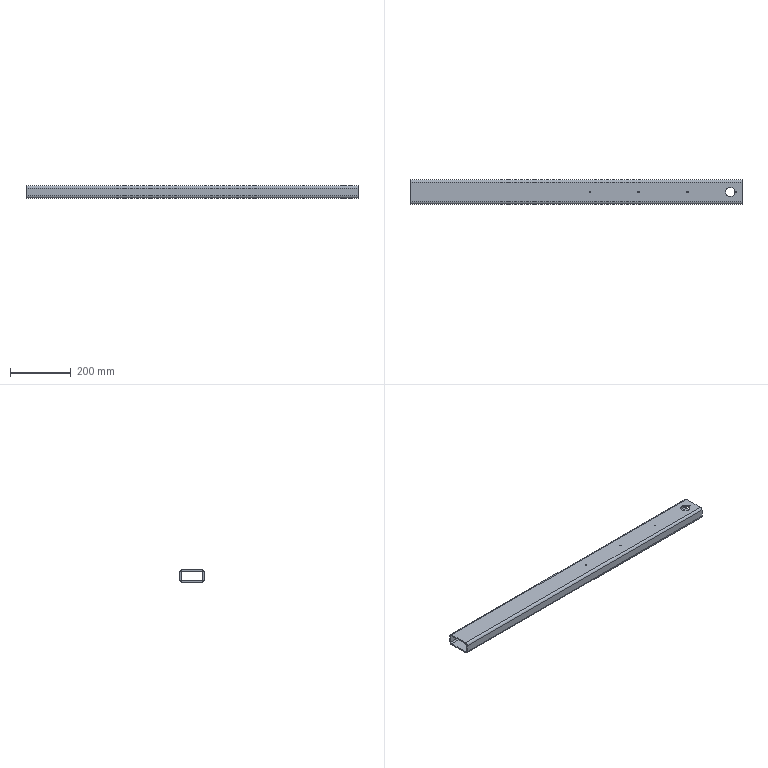Part | SolidWorks | features Cut 1, HoleWzd 1, WeldMemberFeat 1, WeldmentFeature 1 | 1 solid | 38 faces | box 1089 x 80 x 40 mm | volume 924590 mm3 | cylinder 28 | plane 10 | commonest cylinder face diameters 5 x16 8 x4 16 x4 30 x4
STEP:
#1=CARTESIAN_POINT('',(1036.,0.,-20.));
#2=VERTEX_POINT('',#1);
#3=CARTESIAN_POINT('',(1066.,0.,-20.));
#4=VERTEX_POINT('',#3);
#5=CARTESIAN_POINT('',(1051.,0.,-20.));
#6=DIRECTION('',(0.,0.,1.));
#7=DIRECTION('',(1.,0.,0.));
#8=AXIS2_PLACEMENT_3D('',#5,#6,#7);
#9=CIRCLE('',#8,15.);
#10=EDGE_CURVE('',#2,#4,#9,.T.);
#11=ORIENTED_EDGE('',*,*,#10,.F.);
#12=CARTESIAN_POINT('',(1036.,0.,-16.));
#13=VERTEX_POINT('',#12);
#14=CARTESIAN_POINT('',(1036.,0.,-20.));
#15=DIRECTION('',(0.,0.,1.));
#16=VECTOR('',#15,1000.);
#17=LINE('',#14,#16);
#18=EDGE_CURVE('',#2,#13,#17,.T.);
#19=ORIENTED_EDGE('',*,*,#18,.T.);
#20=CARTESIAN_POINT('',(1066.,0.,-16.));
#21=VERTEX_POINT('',#20);
#22=CARTESIAN_POINT('',(1051.,0.,-16.));
#23=DIRECTION('',(0.,0.,1.));
#24=DIRECTION('',(1.,0.,0.));
#25=AXIS2_PLACEMENT_3D('',#22,#23,#24);
#26=CIRCLE('',#25,15.);
#27=EDGE_CURVE('',#13,#21,#26,.T.);
#28=ORIENTED_EDGE('',*,*,#27,.T.);
#29=CARTESIAN_POINT('',(1066.,0.,-20.));
#30=DIRECTION('',(0.,0.,1.));
#31=VECTOR('',#30,1000.);
#32=LINE('',#29,#31);
#33=EDGE_CURVE('',#4,#21,#32,.T.);
#34=ORIENTED_EDGE('',*,*,#33,.F.);
#35=EDGE_LOOP('',(#11,#19,#28,#34));
#36=FACE_OUTER_BOUND('',#35,.T.);
#37=CARTESIAN_POINT('',(1051.,0.,-20.));
#38=DIRECTION('',(0.,0.,1.));
#39=DIRECTION('',(1.,0.,0.));
#40=AXIS2_PLACEMENT_3D('',#37,#38,#39);
#41=CYLINDRICAL_SURFACE('',#40,15.);
#42=ADVANCED_FACE('',(#36),#41,.F.);
#43=CARTESIAN_POINT('',(1066.,0.,16.));
#44=VERTEX_POINT('',#43);
#45=CARTESIAN_POINT('',(1036.,0.,16.));
#46=VERTEX_POINT('',#45);
#47=CARTESIAN_POINT('',(1051.,0.,16.));
#48=DIRECTION('',(0.,0.,-1.));
#49=DIRECTION('',(-1.,0.,0.));
#50=AXIS2_PLACEMENT_3D('',#47,#48,#49);
#51=CIRCLE('',#50,15.);
#52=EDGE_CURVE('',#44,#46,#51,.T.);
#53=ORIENTED_EDGE('',*,*,#52,.T.);
#54=CARTESIAN_POINT('',(1036.,0.,20.));
#55=VERTEX_POINT('',#54);
#56=CARTESIAN_POINT('',(1036.,0.,-20.));
#57=DIRECTION('',(0.,0.,1.));
#58=VECTOR('',#57,1000.);
#59=LINE('',#56,#58);
#60=EDGE_CURVE('',#46,#55,#59,.T.);
#61=ORIENTED_EDGE('',*,*,#60,.T.);
#62=CARTESIAN_POINT('',(1066.,0.,20.));
#63=VERTEX_POINT('',#62);
#64=CARTESIAN_POINT('',(1051.,0.,20.));
#65=DIRECTION('',(0.,0.,1.));
#66=DIRECTION('',(1.,0.,0.));
#67=AXIS2_PLACEMENT_3D('',#64,#65,#66);
#68=CIRCLE('',#67,15.);
#69=EDGE_CURVE('',#55,#63,#68,.T.);
#70=ORIENTED_EDGE('',*,*,#69,.T.);
#71=CARTESIAN_POINT('',(1066.,0.,-20.));
#72=DIRECTION('',(0.,0.,1.));
#73=VECTOR('',#72,1000.);
#74=LINE('',#71,#73);
#75=EDGE_CURVE('',#44,#63,#74,.T.);
#76=ORIENTED_EDGE('',*,*,#75,.F.);
#77=EDGE_LOOP('',(#53,#61,#70,#76));
#78=FACE_OUTER_BOUND('',#77,.T.);
#79=CARTESIAN_POINT('',(1051.,0.,-20.));
#80=DIRECTION('',(0.,0.,1.));
#81=DIRECTION('',(1.,0.,0.));
#82=AXIS2_PLACEMENT_3D('',#79,#80,#81);
#83=CYLINDRICAL_SURFACE('',#82,15.);
#84=ADVANCED_FACE('',(#78),#83,.F.);
#85=CARTESIAN_POINT('',(587.5,0.,-16.));
#86=VERTEX_POINT('',#85);
#87=CARTESIAN_POINT('',(592.5,0.,-16.));
#88=VERTEX_POINT('',#87);
#89=CARTESIAN_POINT('',(590.,0.,-16.));
#90=DIRECTION('',(0.,0.,1.));
#91=DIRECTION('',(1.,0.,0.));
#92=AXIS2_PLACEMENT_3D('',#89,#90,#91);
#93=CIRCLE('',#92,2.5);
#94=EDGE_CURVE('',#86,#88,#93,.T.);
#95=ORIENTED_EDGE('',*,*,#94,.T.);
#96=CARTESIAN_POINT('',(592.5,0.,-20.));
#97=VERTEX_POINT('',#96);
#98=CARTESIAN_POINT('',(592.5,0.,-20.));
#99=DIRECTION('',(0.,0.,-1.));
#100=VECTOR('',#99,1000.);
#101=LINE('',#98,#100);
#102=EDGE_CURVE('',#88,#97,#101,.T.);
#103=ORIENTED_EDGE('',*,*,#102,.T.);
#104=CARTESIAN_POINT('',(587.5,0.,-20.));
#105=VERTEX_POINT('',#104);
#106=CARTESIAN_POINT('',(590.,0.,-20.));
#107=DIRECTION('',(0.,0.,-1.));
#108=DIRECTION('',(-1.,0.,0.));
#109=AXIS2_PLACEMENT_3D('',#106,#107,#108);
#110=CIRCLE('',#109,2.5);
#111=EDGE_CURVE('',#97,#105,#110,.T.);
#112=ORIENTED_EDGE('',*,*,#111,.T.);
#113=CARTESIAN_POINT('',(587.5,0.,-20.));
#114=DIRECTION('',(0.,0.,-1.));
#115=VECTOR('',#114,1000.);
#116=LINE('',#113,#115);
#117=EDGE_CURVE('',#86,#105,#116,.T.);
#118=ORIENTED_EDGE('',*,*,#117,.F.);
#119=EDGE_LOOP('',(#95,#103,#112,#118));
#120=FACE_OUTER_BOUND('',#119,.T.);
#121=CARTESIAN_POINT('',(590.,0.,-20.));
#122=DIRECTION('',(0.,0.,-1.));
#123=DIRECTION('',(-1.,0.,0.));
#124=AXIS2_PLACEMENT_3D('',#121,#122,#123);
#125=CYLINDRICAL_SURFACE('',#124,2.5);
#126=ADVANCED_FACE('',(#120),#125,.F.);
#127=CARTESIAN_POINT('',(592.5,0.,20.));
#128=VERTEX_POINT('',#127);
#129=CARTESIAN_POINT('',(587.5,0.,20.));
#130=VERTEX_POINT('',#129);
#131=CARTESIAN_POINT('',(590.,0.,20.));
#132=DIRECTION('',(0.,0.,-1.));
#133=DIRECTION('',(-1.,0.,0.));
#134=AXIS2_PLACEMENT_3D('',#131,#132,#133);
#135=CIRCLE('',#134,2.5);
#136=EDGE_CURVE('',#128,#130,#135,.T.);
#137=ORIENTED_EDGE('',*,*,#136,.F.);
#138=CARTESIAN_POINT('',(592.5,0.,16.));
#139=VERTEX_POINT('',#138);
#140=CARTESIAN_POINT('',(592.5,0.,-20.));
#141=DIRECTION('',(0.,0.,-1.));
#142=VECTOR('',#141,1000.);
#143=LINE('',#140,#142);
#144=EDGE_CURVE('',#128,#139,#143,.T.);
#145=ORIENTED_EDGE('',*,*,#144,.T.);
#146=CARTESIAN_POINT('',(587.5,0.,16.));
#147=VERTEX_POINT('',#146);
#148=CARTESIAN_POINT('',(590.,0.,16.));
#149=DIRECTION('',(0.,0.,-1.));
#150=DIRECTION('',(-1.,0.,0.));
#151=AXIS2_PLACEMENT_3D('',#148,#149,#150);
#152=CIRCLE('',#151,2.5);
#153=EDGE_CURVE('',#139,#147,#152,.T.);
#154=ORIENTED_EDGE('',*,*,#153,.T.);
#155=CARTESIAN_POINT('',(587.5,0.,-20.));
#156=DIRECTION('',(0.,0.,-1.));
#157=VECTOR('',#156,1000.);
#158=LINE('',#155,#157);
#159=EDGE_CURVE('',#130,#147,#158,.T.);
#160=ORIENTED_EDGE('',*,*,#159,.F.);
#161=EDGE_LOOP('',(#137,#145,#154,#160));
#162=FACE_OUTER_BOUND('',#161,.T.);
#163=CARTESIAN_POINT('',(590.,0.,-20.));
#164=DIRECTION('',(0.,0.,-1.));
#165=DIRECTION('',(-1.,0.,0.));
#166=AXIS2_PLACEMENT_3D('',#163,#164,#165);
#167=CYLINDRICAL_SURFACE('',#166,2.5);
#168=ADVANCED_FACE('',(#162),#167,.F.);
#169=CARTESIAN_POINT('',(752.5,0.,20.));
#170=VERTEX_POINT('',#169);
#171=CARTESIAN_POINT('',(747.5,0.,20.));
#172=VERTEX_POINT('',#171);
#173=CARTESIAN_POINT('',(750.,0.,20.));
#174=DIRECTION('',(0.,0.,-1.));
#175=DIRECTION('',(-1.,0.,0.));
#176=AXIS2_PLACEMENT_3D('',#173,#174,#175);
#177=CIRCLE('',#176,2.5);
#178=EDGE_CURVE('',#170,#172,#177,.T.);
#179=ORIENTED_EDGE('',*,*,#178,.F.);
#180=CARTESIAN_POINT('',(752.5,0.,16.));
#181=VERTEX_POINT('',#180);
#182=CARTESIAN_POINT('',(752.5,0.,-20.));
#183=DIRECTION('',(0.,0.,-1.));
#184=VECTOR('',#183,1000.);
#185=LINE('',#182,#184);
#186=EDGE_CURVE('',#170,#181,#185,.T.);
#187=ORIENTED_EDGE('',*,*,#186,.T.);
#188=CARTESIAN_POINT('',(747.5,0.,16.));
#189=VERTEX_POINT('',#188);
#190=CARTESIAN_POINT('',(750.,0.,16.));
#191=DIRECTION('',(0.,0.,-1.));
#192=DIRECTION('',(-1.,0.,0.));
#193=AXIS2_PLACEMENT_3D('',#190,#191,#192);
#194=CIRCLE('',#193,2.5);
#195=EDGE_CURVE('',#181,#189,#194,.T.);
#196=ORIENTED_EDGE('',*,*,#195,.T.);
#197=CARTESIAN_POINT('',(747.5,0.,-20.));
#198=DIRECTION('',(0.,0.,-1.));
#199=VECTOR('',#198,1000.);
#200=LINE('',#197,#199);
#201=EDGE_CURVE('',#172,#189,#200,.T.);
#202=ORIENTED_EDGE('',*,*,#201,.F.);
#203=EDGE_LOOP('',(#179,#187,#196,#202));
#204=FACE_OUTER_BOUND('',#203,.T.);
#205=CARTESIAN_POINT('',(750.,0.,-20.));
#206=DIRECTION('',(0.,0.,-1.));
#207=DIRECTION('',(-1.,0.,0.));
#208=AXIS2_PLACEMENT_3D('',#205,#206,#207);
#209=CYLINDRICAL_SURFACE('',#208,2.5);
#210=ADVANCED_FACE('',(#204),#209,.F.);
#211=CARTESIAN_POINT('',(747.5,0.,-16.));
#212=VERTEX_POINT('',#211);
#213=CARTESIAN_POINT('',(752.5,0.,-16.));
#214=VERTEX_POINT('',#213);
#215=CARTESIAN_POINT('',(750.,0.,-16.));
#216=DIRECTION('',(0.,0.,1.));
#217=DIRECTION('',(1.,0.,0.));
#218=AXIS2_PLACEMENT_3D('',#215,#216,#217);
#219=CIRCLE('',#218,2.5);
#220=EDGE_CURVE('',#212,#214,#219,.T.);
#221=ORIENTED_EDGE('',*,*,#220,.T.);
#222=CARTESIAN_POINT('',(752.5,0.,-20.));
#223=VERTEX_POINT('',#222);
#224=CARTESIAN_POINT('',(752.5,0.,-20.));
#225=DIRECTION('',(0.,0.,-1.));
#226=VECTOR('',#225,1000.);
#227=LINE('',#224,#226);
#228=EDGE_CURVE('',#214,#223,#227,.T.);
#229=ORIENTED_EDGE('',*,*,#228,.T.);
#230=CARTESIAN_POINT('',(747.5,0.,-20.));
#231=VERTEX_POINT('',#230);
#232=CARTESIAN_POINT('',(750.,0.,-20.));
#233=DIRECTION('',(0.,0.,-1.));
#234=DIRECTION('',(-1.,0.,0.));
#235=AXIS2_PLACEMENT_3D('',#232,#233,#234);
#236=CIRCLE('',#235,2.5);
#237=EDGE_CURVE('',#223,#231,#236,.T.);
#238=ORIENTED_EDGE('',*,*,#237,.T.);
#239=CARTESIAN_POINT('',(747.5,0.,-20.));
#240=DIRECTION('',(0.,0.,-1.));
#241=VECTOR('',#240,1000.);
#242=LINE('',#239,#241);
#243=EDGE_CURVE('',#212,#231,#242,.T.);
#244=ORIENTED_EDGE('',*,*,#243,.F.);
#245=EDGE_LOOP('',(#221,#229,#238,#244));
#246=FACE_OUTER_BOUND('',#245,.T.);
#247=CARTESIAN_POINT('',(750.,0.,-20.));
#248=DIRECTION('',(0.,0.,-1.));
#249=DIRECTION('',(-1.,0.,0.));
#250=AXIS2_PLACEMENT_3D('',#247,#248,#249);
#251=CYLINDRICAL_SURFACE('',#250,2.5);
#252=ADVANCED_FACE('',(#246),#251,.F.);
#253=CARTESIAN_POINT('',(907.5,0.,-16.));
#254=VERTEX_POINT('',#253);
#255=CARTESIAN_POINT('',(912.5,0.,-16.));
#256=VERTEX_POINT('',#255);
#257=CARTESIAN_POINT('',(910.,0.,-16.));
#258=DIRECTION('',(0.,0.,1.));
#259=DIRECTION('',(1.,0.,0.));
#260=AXIS2_PLACEMENT_3D('',#257,#258,#259);
#261=CIRCLE('',#260,2.5);
#262=EDGE_CURVE('',#254,#256,#261,.T.);
#263=ORIENTED_EDGE('',*,*,#262,.T.);
#264=CARTESIAN_POINT('',(912.5,0.,-20.));
#265=VERTEX_POINT('',#264);
#266=CARTESIAN_POINT('',(912.5,0.,-20.));
#267=DIRECTION('',(0.,0.,-1.));
#268=VECTOR('',#267,1000.);
#269=LINE('',#266,#268);
#270=EDGE_CURVE('',#256,#265,#269,.T.);
#271=ORIENTED_EDGE('',*,*,#270,.T.);
#272=CARTESIAN_POINT('',(907.5,0.,-20.));
#273=VERTEX_POINT('',#272);
#274=CARTESIAN_POINT('',(910.,0.,-20.));
#275=DIRECTION('',(0.,0.,-1.));
#276=DIRECTION('',(-1.,0.,0.));
#277=AXIS2_PLACEMENT_3D('',#274,#275,#276);
#278=CIRCLE('',#277,2.5);
#279=EDGE_CURVE('',#265,#273,#278,.T.);
#280=ORIENTED_EDGE('',*,*,#279,.T.);
#281=CARTESIAN_POINT('',(907.5,0.,-20.));
#282=DIRECTION('',(0.,0.,-1.));
#283=VECTOR('',#282,1000.);
#284=LINE('',#281,#283);
#285=EDGE_CURVE('',#254,#273,#284,.T.);
#286=ORIENTED_EDGE('',*,*,#285,.F.);
#287=EDGE_LOOP('',(#263,#271,#280,#286));
#288=FACE_OUTER_BOUND('',#287,.T.);
#289=CARTESIAN_POINT('',(910.,0.,-20.));
#290=DIRECTION('',(0.,0.,-1.));
#291=DIRECTION('',(-1.,0.,0.));
#292=AXIS2_PLACEMENT_3D('',#289,#290,#291);
#293=CYLINDRICAL_SURFACE('',#292,2.5);
#294=ADVANCED_FACE('',(#288),#293,.F.);
#295=CARTESIAN_POINT('',(912.5,0.,20.));
#296=VERTEX_POINT('',#295);
#297=CARTESIAN_POINT('',(907.5,0.,20.));
#298=VERTEX_POINT('',#297);
#299=CARTESIAN_POINT('',(910.,0.,20.));
#300=DIRECTION('',(0.,0.,-1.));
#301=DIRECTION('',(-1.,0.,0.));
#302=AXIS2_PLACEMENT_3D('',#299,#300,#301);
#303=CIRCLE('',#302,2.5);
#304=EDGE_CURVE('',#296,#298,#303,.T.);
#305=ORIENTED_EDGE('',*,*,#304,.F.);
#306=CARTESIAN_POINT('',(912.5,0.,16.));
#307=VERTEX_POINT('',#306);
#308=CARTESIAN_POINT('',(912.5,0.,-20.));
#309=DIRECTION('',(0.,0.,-1.));
#310=VECTOR('',#309,1000.);
#311=LINE('',#308,#310);
#312=EDGE_CURVE('',#296,#307,#311,.T.);
#313=ORIENTED_EDGE('',*,*,#312,.T.);
#314=CARTESIAN_POINT('',(907.5,0.,16.));
#315=VERTEX_POINT('',#314);
#316=CARTESIAN_POINT('',(910.,0.,16.));
#317=DIRECTION('',(0.,0.,-1.));
#318=DIRECTION('',(-1.,0.,0.));
#319=AXIS2_PLACEMENT_3D('',#316,#317,#318);
#320=CIRCLE('',#319,2.5);
#321=EDGE_CURVE('',#307,#315,#320,.T.);
#322=ORIENTED_EDGE('',*,*,#321,.T.);
#323=CARTESIAN_POINT('',(907.5,0.,-20.));
#324=DIRECTION('',(0.,0.,-1.));
#325=VECTOR('',#324,1000.);
#326=LINE('',#323,#325);
#327=EDGE_CURVE('',#298,#315,#326,.T.);
#328=ORIENTED_EDGE('',*,*,#327,.F.);
#329=EDGE_LOOP('',(#305,#313,#322,#328));
#330=FACE_OUTER_BOUND('',#329,.T.);
#331=CARTESIAN_POINT('',(910.,0.,-20.));
#332=DIRECTION('',(0.,0.,-1.));
#333=DIRECTION('',(-1.,0.,0.));
#334=AXIS2_PLACEMENT_3D('',#331,#332,#333);
#335=CYLINDRICAL_SURFACE('',#334,2.5);
#336=ADVANCED_FACE('',(#330),#335,.F.);
#337=CARTESIAN_POINT('',(1072.5,0.,20.));
#338=VERTEX_POINT('',#337);
#339=CARTESIAN_POINT('',(1067.5,0.,20.));
#340=VERTEX_POINT('',#339);
#341=CARTESIAN_POINT('',(1070.,0.,20.));
#342=DIRECTION('',(0.,0.,-1.));
#343=DIRECTION('',(-1.,0.,0.));
#344=AXIS2_PLACEMENT_3D('',#341,#342,#343);
#345=CIRCLE('',#344,2.5);
#346=EDGE_CURVE('',#338,#340,#345,.T.);
#347=ORIENTED_EDGE('',*,*,#346,.F.);
#348=CARTESIAN_POINT('',(1072.5,0.,16.));
#349=VERTEX_POINT('',#348);
#350=CARTESIAN_POINT('',(1072.5,0.,-20.));
#351=DIRECTION('',(0.,0.,-1.));
#352=VECTOR('',#351,1000.);
#353=LINE('',#350,#352);
#354=EDGE_CURVE('',#338,#349,#353,.T.);
#355=ORIENTED_EDGE('',*,*,#354,.T.);
#356=CARTESIAN_POINT('',(1067.5,0.,16.));
#357=VERTEX_POINT('',#356);
#358=CARTESIAN_POINT('',(1070.,0.,16.));
#359=DIRECTION('',(0.,0.,-1.));
#360=DIRECTION('',(-1.,0.,0.));
#361=AXIS2_PLACEMENT_3D('',#358,#359,#360);
#362=CIRCLE('',#361,2.5);
#363=EDGE_CURVE('',#349,#357,#362,.T.);
#364=ORIENTED_EDGE('',*,*,#363,.T.);
#365=CARTESIAN_POINT('',(1067.5,0.,-20.));
#366=DIRECTION('',(0.,0.,-1.));
#367=VECTOR('',#366,1000.);
#368=LINE('',#365,#367);
#369=EDGE_CURVE('',#340,#357,#368,.T.);
#370=ORIENTED_EDGE('',*,*,#369,.F.);
#371=EDGE_LOOP('',(#347,#355,#364,#370));
#372=FACE_OUTER_BOUND('',#371,.T.);
#373=CARTESIAN_POINT('',(1070.,0.,-20.));
#374=DIRECTION('',(0.,0.,-1.));
#375=DIRECTION('',(-1.,0.,0.));
#376=AXIS2_PLACEMENT_3D('',#373,#374,#375);
#377=CYLINDRICAL_SURFACE('',#376,2.5);
#378=ADVANCED_FACE('',(#372),#377,.F.);
#379=CARTESIAN_POINT('',(1067.5,0.,-16.));
#380=VERTEX_POINT('',#379);
#381=CARTESIAN_POINT('',(1072.5,0.,-16.));
#382=VERTEX_POINT('',#381);
#383=CARTESIAN_POINT('',(1070.,0.,-16.));
#384=DIRECTION('',(0.,0.,1.));
#385=DIRECTION('',(1.,0.,0.));
#386=AXIS2_PLACEMENT_3D('',#383,#384,#385);
#387=CIRCLE('',#386,2.5);
#388=EDGE_CURVE('',#380,#382,#387,.T.);
#389=ORIENTED_EDGE('',*,*,#388,.T.);
#390=CARTESIAN_POINT('',(1072.5,0.,-20.));
#391=VERTEX_POINT('',#390);
#392=CARTESIAN_POINT('',(1072.5,0.,-20.));
#393=DIRECTION('',(0.,0.,-1.));
#394=VECTOR('',#393,1000.);
#395=LINE('',#392,#394);
#396=EDGE_CURVE('',#382,#391,#395,.T.);
#397=ORIENTED_EDGE('',*,*,#396,.T.);
#398=CARTESIAN_POINT('',(1067.5,0.,-20.));
#399=VERTEX_POINT('',#398);
#400=CARTESIAN_POINT('',(1070.,0.,-20.));
#401=DIRECTION('',(0.,0.,-1.));
#402=DIRECTION('',(-1.,0.,0.));
#403=AXIS2_PLACEMENT_3D('',#400,#401,#402);
#404=CIRCLE('',#403,2.5);
#405=EDGE_CURVE('',#391,#399,#404,.T.);
#406=ORIENTED_EDGE('',*,*,#405,.T.);
#407=CARTESIAN_POINT('',(1067.5,0.,-20.));
#408=DIRECTION('',(0.,0.,-1.));
#409=VECTOR('',#408,1000.);
#410=LINE('',#407,#409);
#411=EDGE_CURVE('',#380,#399,#410,.T.);
#412=ORIENTED_EDGE('',*,*,#411,.F.);
#413=EDGE_LOOP('',(#389,#397,#406,#412));
#414=FACE_OUTER_BOUND('',#413,.T.);
#415=CARTESIAN_POINT('',(1070.,0.,-20.));
#416=DIRECTION('',(0.,0.,-1.));
#417=DIRECTION('',(-1.,0.,0.));
#418=AXIS2_PLACEMENT_3D('',#415,#416,#417);
#419=CYLINDRICAL_SURFACE('',#418,2.5);
#420=ADVANCED_FACE('',(#414),#419,.F.);
#421=CARTESIAN_POINT('',(1051.,0.,-20.));
#422=DIRECTION('',(0.,0.,1.));
#423=DIRECTION('',(1.,0.,0.));
#424=AXIS2_PLACEMENT_3D('',#421,#422,#423);
#425=CIRCLE('',#424,15.);
#426=EDGE_CURVE('',#4,#2,#425,.T.);
#427=ORIENTED_EDGE('',*,*,#426,.T.);
#428=ORIENTED_EDGE('',*,*,#10,.T.);
#429=EDGE_LOOP('',(#427,#428));
#430=FACE_BOUND('',#429,.T.);
#431=CARTESIAN_POINT('',(750.,0.,-20.));
#432=DIRECTION('',(0.,0.,-1.));
#433=DIRECTION('',(-1.,0.,0.));
#434=AXIS2_PLACEMENT_3D('',#431,#432,#433);
#435=CIRCLE('',#434,2.5);
#436=EDGE_CURVE('',#231,#223,#435,.T.);
#437=ORIENTED_EDGE('',*,*,#436,.F.);
#438=ORIENTED_EDGE('',*,*,#237,.F.);
#439=EDGE_LOOP('',(#437,#438));
#440=FACE_BOUND('',#439,.T.);
#441=CARTESIAN_POINT('',(910.,0.,-20.));
#442=DIRECTION('',(0.,0.,-1.));
#443=DIRECTION('',(-1.,0.,0.));
#444=AXIS2_PLACEMENT_3D('',#441,#442,#443);
#445=CIRCLE('',#444,2.5);
#446=EDGE_CURVE('',#273,#265,#445,.T.);
#447=ORIENTED_EDGE('',*,*,#446,.F.);
#448=ORIENTED_EDGE('',*,*,#279,.F.);
#449=EDGE_LOOP('',(#447,#448));
#450=FACE_BOUND('',#449,.T.);
#451=CARTESIAN_POINT('',(1070.,0.,-20.));
#452=DIRECTION('',(0.,0.,-1.));
#453=DIRECTION('',(-1.,0.,0.));
#454=AXIS2_PLACEMENT_3D('',#451,#452,#453);
#455=CIRCLE('',#454,2.5);
#456=EDGE_CURVE('',#399,#391,#455,.T.);
#457=ORIENTED_EDGE('',*,*,#456,.F.);
#458=ORIENTED_EDGE('',*,*,#405,.F.);
#459=EDGE_LOOP('',(#457,#458));
#460=FACE_BOUND('',#459,.T.);
#461=CARTESIAN_POINT('',(0.,-32.,-20.));
#462=VERTEX_POINT('',#461);
#463=CARTESIAN_POINT('',(0.,32.,-20.));
#464=VERTEX_POINT('',#463);
#465=CARTESIAN_POINT('',(0.,32.,-20.));
#466=DIRECTION('',(0.,1.,0.));
#467=VECTOR('',#466,1000.);
#468=LINE('',#465,#467);
#469=EDGE_CURVE('',#462,#464,#468,.T.);
#470=ORIENTED_EDGE('',*,*,#469,.T.);
#471=CARTESIAN_POINT('',(1089.,32.,-20.));
#472=VERTEX_POINT('',#471);
#473=CARTESIAN_POINT('',(1089.,32.,-20.));
#474=DIRECTION('',(-1.,0.,0.));
#475=VECTOR('',#474,1000.);
#476=LINE('',#473,#475);
#477=EDGE_CURVE('',#472,#464,#476,.T.);
#478=ORIENTED_EDGE('',*,*,#477,.F.);
#479=CARTESIAN_POINT('',(1089.,-32.,-20.));
#480=VERTEX_POINT('',#479);
#481=CARTESIAN_POINT('',(1089.,32.,-20.));
#482=DIRECTION('',(0.,1.,0.));
#483=VECTOR('',#482,1000.);
#484=LINE('',#481,#483);
#485=EDGE_CURVE('',#480,#472,#484,.T.);
#486=ORIENTED_EDGE('',*,*,#485,.F.);
#487=CARTESIAN_POINT('',(1089.,-32.,-20.));
#488=DIRECTION('',(-1.,0.,0.));
#489=VECTOR('',#488,1000.);
#490=LINE('',#487,#489);
#491=EDGE_CURVE('',#480,#462,#490,.T.);
#492=ORIENTED_EDGE('',*,*,#491,.T.);
#493=EDGE_LOOP('',(#470,#478,#486,#492));
#494=FACE_OUTER_BOUND('',#493,.T.);
#495=CARTESIAN_POINT('',(590.,0.,-20.));
#496=DIRECTION('',(0.,0.,-1.));
#497=DIRECTION('',(-1.,0.,0.));
#498=AXIS2_PLACEMENT_3D('',#495,#496,#497);
#499=CIRCLE('',#498,2.5);
#500=EDGE_CURVE('',#105,#97,#499,.T.);
#501=ORIENTED_EDGE('',*,*,#500,.F.);
#502=ORIENTED_EDGE('',*,*,#111,.F.);
#503=EDGE_LOOP('',(#501,#502));
#504=FACE_BOUND('',#503,.T.);
#505=CARTESIAN_POINT('',(1089.,32.,-20.));
#506=DIRECTION('',(0.,0.,1.));
#507=DIRECTION('',(1.,0.,0.));
#508=AXIS2_PLACEMENT_3D('',#505,#506,#507);
#509=PLANE('',#508);
#510=ADVANCED_FACE('',(#430,#440,#450,#460,#494,#504),#509,.F.);
#511=CARTESIAN_POINT('',(0.,40.,-12.));
#512=VERTEX_POINT('',#511);
#513=CARTESIAN_POINT('',(0.,32.,-12.));
#514=DIRECTION('',(1.,0.,0.));
#515=DIRECTION('',(0.,0.,-1.));
#516=AXIS2_PLACEMENT_3D('',#513,#514,#515);
#517=CIRCLE('',#516,8.);
#518=EDGE_CURVE('',#464,#512,#517,.T.);
#519=ORIENTED_EDGE('',*,*,#518,.T.);
#520=CARTESIAN_POINT('',(1089.,40.,-12.));
#521=VERTEX_POINT('',#520);
#522=CARTESIAN_POINT('',(1089.,40.,-12.));
#523=DIRECTION('',(-1.,0.,0.));
#524=VECTOR('',#523,1000.);
#525=LINE('',#522,#524);
#526=EDGE_CURVE('',#521,#512,#525,.T.);
#527=ORIENTED_EDGE('',*,*,#526,.F.);
#528=CARTESIAN_POINT('',(1089.,32.,-12.));
#529=DIRECTION('',(1.,0.,0.));
#530=DIRECTION('',(0.,0.,-1.));
#531=AXIS2_PLACEMENT_3D('',#528,#529,#530);
#532=CIRCLE('',#531,8.);
#533=EDGE_CURVE('',#472,#521,#532,.T.);
#534=ORIENTED_EDGE('',*,*,#533,.F.);
#535=ORIENTED_EDGE('',*,*,#477,.T.);
#536=EDGE_LOOP('',(#519,#527,#534,#535));
#537=FACE_OUTER_BOUND('',#536,.T.);
#538=CARTESIAN_POINT('',(1089.,32.,-12.));
#539=DIRECTION('',(-1.,0.,0.));
#540=DIRECTION('',(0.,0.,1.));
#541=AXIS2_PLACEMENT_3D('',#538,#539,#540);
#542=CYLINDRICAL_SURFACE('',#541,8.);
#543=ADVANCED_FACE('',(#537),#542,.T.);
#544=CARTESIAN_POINT('',(0.,40.,12.));
#545=VERTEX_POINT('',#544);
#546=CARTESIAN_POINT('',(0.,40.,-12.));
#547=DIRECTION('',(0.,0.,1.));
#548=VECTOR('',#547,1000.);
#549=LINE('',#546,#548);
#550=EDGE_CURVE('',#512,#545,#549,.T.);
#551=ORIENTED_EDGE('',*,*,#550,.T.);
#552=CARTESIAN_POINT('',(1089.,40.,12.));
#553=VERTEX_POINT('',#552);
#554=CARTESIAN_POINT('',(1089.,40.,12.));
#555=DIRECTION('',(-1.,0.,0.));
#556=VECTOR('',#555,1000.);
#557=LINE('',#554,#556);
#558=EDGE_CURVE('',#553,#545,#557,.T.);
#559=ORIENTED_EDGE('',*,*,#558,.F.);
#560=CARTESIAN_POINT('',(1089.,40.,-12.));
#561=DIRECTION('',(0.,0.,1.));
#562=VECTOR('',#561,1000.);
#563=LINE('',#560,#562);
#564=EDGE_CURVE('',#521,#553,#563,.T.);
#565=ORIENTED_EDGE('',*,*,#564,.F.);
#566=ORIENTED_EDGE('',*,*,#526,.T.);
#567=EDGE_LOOP('',(#551,#559,#565,#566));
#568=FACE_OUTER_BOUND('',#567,.T.);
#569=CARTESIAN_POINT('',(1089.,40.,-12.));
#570=DIRECTION('',(0.,-1.,0.));
#571=DIRECTION('',(0.,0.,-1.));
#572=AXIS2_PLACEMENT_3D('',#569,#570,#571);
#573=PLANE('',#572);
#574=ADVANCED_FACE('',(#568),#573,.F.);
#575=CARTESIAN_POINT('',(0.,32.,20.));
#576=VERTEX_POINT('',#575);
#577=CARTESIAN_POINT('',(0.,32.,12.));
#578=DIRECTION('',(1.,0.,0.));
#579=DIRECTION('',(0.,0.,-1.));
#580=AXIS2_PLACEMENT_3D('',#577,#578,#579);
#581=CIRCLE('',#580,8.);
#582=EDGE_CURVE('',#545,#576,#581,.T.);
#583=ORIENTED_EDGE('',*,*,#582,.T.);
#584=CARTESIAN_POINT('',(1089.,32.,20.));
#585=VERTEX_POINT('',#584);
#586=CARTESIAN_POINT('',(1089.,32.,20.));
#587=DIRECTION('',(-1.,0.,0.));
#588=VECTOR('',#587,1000.);
#589=LINE('',#586,#588);
#590=EDGE_CURVE('',#585,#576,#589,.T.);
#591=ORIENTED_EDGE('',*,*,#590,.F.);
#592=CARTESIAN_POINT('',(1089.,32.,12.));
#593=DIRECTION('',(1.,0.,0.));
#594=DIRECTION('',(0.,0.,-1.));
#595=AXIS2_PLACEMENT_3D('',#592,#593,#594);
#596=CIRCLE('',#595,8.);
#597=EDGE_CURVE('',#553,#585,#596,.T.);
#598=ORIENTED_EDGE('',*,*,#597,.F.);
#599=ORIENTED_EDGE('',*,*,#558,.T.);
#600=EDGE_LOOP('',(#583,#591,#598,#599));
#601=FACE_OUTER_BOUND('',#600,.T.);
#602=CARTESIAN_POINT('',(1089.,32.,12.));
#603=DIRECTION('',(-1.,0.,0.));
#604=DIRECTION('',(0.,0.,1.));
#605=AXIS2_PLACEMENT_3D('',#602,#603,#604);
#606=CYLINDRICAL_SURFACE('',#605,8.);
#607=ADVANCED_FACE('',(#601),#606,.T.);
#608=CARTESIAN_POINT('',(1051.,0.,20.));
#609=DIRECTION('',(0.,0.,1.));
#610=DIRECTION('',(1.,0.,0.));
#611=AXIS2_PLACEMENT_3D('',#608,#609,#610);
#612=CIRCLE('',#611,15.);
#613=EDGE_CURVE('',#63,#55,#612,.T.);
#614=ORIENTED_EDGE('',*,*,#613,.F.);
#615=ORIENTED_EDGE('',*,*,#69,.F.);
#616=EDGE_LOOP('',(#614,#615));
#617=FACE_BOUND('',#616,.T.);
#618=CARTESIAN_POINT('',(590.,0.,20.));
#619=DIRECTION('',(0.,0.,-1.));
#620=DIRECTION('',(-1.,0.,0.));
#621=AXIS2_PLACEMENT_3D('',#618,#619,#620);
#622=CIRCLE('',#621,2.5);
#623=EDGE_CURVE('',#130,#128,#622,.T.);
#624=ORIENTED_EDGE('',*,*,#623,.T.);
#625=ORIENTED_EDGE('',*,*,#136,.T.);
#626=EDGE_LOOP('',(#624,#625));
#627=FACE_BOUND('',#626,.T.);
#628=CARTESIAN_POINT('',(750.,0.,20.));
#629=DIRECTION('',(0.,0.,-1.));
#630=DIRECTION('',(-1.,0.,0.));
#631=AXIS2_PLACEMENT_3D('',#628,#629,#630);
#632=CIRCLE('',#631,2.5);
#633=EDGE_CURVE('',#172,#170,#632,.T.);
#634=ORIENTED_EDGE('',*,*,#633,.T.);
#635=ORIENTED_EDGE('',*,*,#178,.T.);
#636=EDGE_LOOP('',(#634,#635));
#637=FACE_BOUND('',#636,.T.);
#638=CARTESIAN_POINT('',(910.,0.,20.));
#639=DIRECTION('',(0.,0.,-1.));
#640=DIRECTION('',(-1.,0.,0.));
#641=AXIS2_PLACEMENT_3D('',#638,#639,#640);
#642=CIRCLE('',#641,2.5);
#643=EDGE_CURVE('',#298,#296,#642,.T.);
#644=ORIENTED_EDGE('',*,*,#643,.T.);
#645=ORIENTED_EDGE('',*,*,#304,.T.);
#646=EDGE_LOOP('',(#644,#645));
#647=FACE_BOUND('',#646,.T.);
#648=CARTESIAN_POINT('',(1070.,0.,20.));
#649=DIRECTION('',(0.,0.,-1.));
#650=DIRECTION('',(-1.,0.,0.));
#651=AXIS2_PLACEMENT_3D('',#648,#649,#650);
#652=CIRCLE('',#651,2.5);
#653=EDGE_CURVE('',#340,#338,#652,.T.);
#654=ORIENTED_EDGE('',*,*,#653,.T.);
#655=ORIENTED_EDGE('',*,*,#346,.T.);
#656=EDGE_LOOP('',(#654,#655));
#657=FACE_BOUND('',#656,.T.);
#658=CARTESIAN_POINT('',(0.,-32.,20.));
#659=VERTEX_POINT('',#658);
#660=CARTESIAN_POINT('',(0.,-32.,20.));
#661=DIRECTION('',(0.,-1.,0.));
#662=VECTOR('',#661,1000.);
#663=LINE('',#660,#662);
#664=EDGE_CURVE('',#576,#659,#663,.T.);
#665=ORIENTED_EDGE('',*,*,#664,.T.);
#666=CARTESIAN_POINT('',(1089.,-32.,20.));
#667=VERTEX_POINT('',#666);
#668=CARTESIAN_POINT('',(1089.,-32.,20.));
#669=DIRECTION('',(-1.,0.,0.));
#670=VECTOR('',#669,1000.);
#671=LINE('',#668,#670);
#672=EDGE_CURVE('',#667,#659,#671,.T.);
#673=ORIENTED_EDGE('',*,*,#672,.F.);
#674=CARTESIAN_POINT('',(1089.,-32.,20.));
#675=DIRECTION('',(0.,-1.,0.));
#676=VECTOR('',#675,1000.);
#677=LINE('',#674,#676);
#678=EDGE_CURVE('',#585,#667,#677,.T.);
#679=ORIENTED_EDGE('',*,*,#678,.F.);
#680=ORIENTED_EDGE('',*,*,#590,.T.);
#681=EDGE_LOOP('',(#665,#673,#679,#680));
#682=FACE_OUTER_BOUND('',#681,.T.);
#683=CARTESIAN_POINT('',(1089.,-32.,20.));
#684=DIRECTION('',(0.,0.,-1.));
#685=DIRECTION('',(-1.,0.,0.));
#686=AXIS2_PLACEMENT_3D('',#683,#684,#685);
#687=PLANE('',#686);
#688=ADVANCED_FACE('',(#617,#627,#637,#647,#657,#682),#687,.F.);
#689=CARTESIAN_POINT('',(0.,-40.,12.));
#690=VERTEX_POINT('',#689);
#691=CARTESIAN_POINT('',(0.,-32.,12.));
#692=DIRECTION('',(1.,0.,0.));
#693=DIRECTION('',(0.,0.,-1.));
#694=AXIS2_PLACEMENT_3D('',#691,#692,#693);
#695=CIRCLE('',#694,8.);
#696=EDGE_CURVE('',#659,#690,#695,.T.);
#697=ORIENTED_EDGE('',*,*,#696,.T.);
#698=CARTESIAN_POINT('',(1089.,-40.,12.));
#699=VERTEX_POINT('',#698);
#700=CARTESIAN_POINT('',(1089.,-40.,12.));
#701=DIRECTION('',(-1.,0.,0.));
#702=VECTOR('',#701,1000.);
#703=LINE('',#700,#702);
#704=EDGE_CURVE('',#699,#690,#703,.T.);
#705=ORIENTED_EDGE('',*,*,#704,.F.);
#706=CARTESIAN_POINT('',(1089.,-32.,12.));
#707=DIRECTION('',(1.,0.,0.));
#708=DIRECTION('',(0.,0.,-1.));
#709=AXIS2_PLACEMENT_3D('',#706,#707,#708);
#710=CIRCLE('',#709,8.);
#711=EDGE_CURVE('',#667,#699,#710,.T.);
#712=ORIENTED_EDGE('',*,*,#711,.F.);
#713=ORIENTED_EDGE('',*,*,#672,.T.);
#714=EDGE_LOOP('',(#697,#705,#712,#713));
#715=FACE_OUTER_BOUND('',#714,.T.);
#716=CARTESIAN_POINT('',(1089.,-32.,12.));
#717=DIRECTION('',(-1.,0.,0.));
#718=DIRECTION('',(0.,0.,1.));
#719=AXIS2_PLACEMENT_3D('',#716,#717,#718);
#720=CYLINDRICAL_SURFACE('',#719,8.);
#721=ADVANCED_FACE('',(#715),#720,.T.);
#722=CARTESIAN_POINT('',(0.,-40.,-12.));
#723=VERTEX_POINT('',#722);
#724=CARTESIAN_POINT('',(0.,-40.,12.));
#725=DIRECTION('',(0.,0.,-1.));
#726=VECTOR('',#725,1000.);
#727=LINE('',#724,#726);
#728=EDGE_CURVE('',#690,#723,#727,.T.);
#729=ORIENTED_EDGE('',*,*,#728,.T.);
#730=CARTESIAN_POINT('',(1089.,-40.,-12.));
#731=VERTEX_POINT('',#730);
#732=CARTESIAN_POINT('',(1089.,-40.,-12.));
#733=DIRECTION('',(-1.,0.,0.));
#734=VECTOR('',#733,1000.);
#735=LINE('',#732,#734);
#736=EDGE_CURVE('',#731,#723,#735,.T.);
#737=ORIENTED_EDGE('',*,*,#736,.F.);
#738=CARTESIAN_POINT('',(1089.,-40.,12.));
#739=DIRECTION('',(0.,0.,-1.));
#740=VECTOR('',#739,1000.);
#741=LINE('',#738,#740);
#742=EDGE_CURVE('',#699,#731,#741,.T.);
#743=ORIENTED_EDGE('',*,*,#742,.F.);
#744=ORIENTED_EDGE('',*,*,#704,.T.);
#745=EDGE_LOOP('',(#729,#737,#743,#744));
#746=FACE_OUTER_BOUND('',#745,.T.);
#747=CARTESIAN_POINT('',(1089.,-40.,12.));
#748=DIRECTION('',(0.,1.,0.));
#749=DIRECTION('',(0.,0.,1.));
#750=AXIS2_PLACEMENT_3D('',#747,#748,#749);
#751=PLANE('',#750);
#752=ADVANCED_FACE('',(#746),#751,.F.);
#753=CARTESIAN_POINT('',(0.,-32.,-12.));
#754=DIRECTION('',(1.,0.,0.));
#755=DIRECTION('',(0.,0.,-1.));
#756=AXIS2_PLACEMENT_3D('',#753,#754,#755);
#757=CIRCLE('',#756,8.);
#758=EDGE_CURVE('',#723,#462,#757,.T.);
#759=ORIENTED_EDGE('',*,*,#758,.T.);
#760=ORIENTED_EDGE('',*,*,#491,.F.);
#761=CARTESIAN_POINT('',(1089.,-32.,-12.));
#762=DIRECTION('',(1.,0.,0.));
#763=DIRECTION('',(0.,0.,-1.));
#764=AXIS2_PLACEMENT_3D('',#761,#762,#763);
#765=CIRCLE('',#764,8.);
#766=EDGE_CURVE('',#731,#480,#765,.T.);
#767=ORIENTED_EDGE('',*,*,#766,.F.);
#768=ORIENTED_EDGE('',*,*,#736,.T.);
#769=EDGE_LOOP('',(#759,#760,#767,#768));
#770=FACE_OUTER_BOUND('',#769,.T.);
#771=CARTESIAN_POINT('',(1089.,-32.,-12.));
#772=DIRECTION('',(-1.,0.,0.));
#773=DIRECTION('',(0.,0.,1.));
#774=AXIS2_PLACEMENT_3D('',#771,#772,#773);
#775=CYLINDRICAL_SURFACE('',#774,8.);
#776=ADVANCED_FACE('',(#770),#775,.T.);
#777=CARTESIAN_POINT('',(0.,36.,12.));
#778=VERTEX_POINT('',#777);
#779=CARTESIAN_POINT('',(0.,32.,16.));
#780=VERTEX_POINT('',#779);
#781=CARTESIAN_POINT('',(0.,32.,12.));
#782=DIRECTION('',(1.,0.,0.));
#783=DIRECTION('',(0.,0.,-1.));
#784=AXIS2_PLACEMENT_3D('',#781,#782,#783);
#785=CIRCLE('',#784,4.);
#786=EDGE_CURVE('',#778,#780,#785,.T.);
#787=ORIENTED_EDGE('',*,*,#786,.F.);
#788=CARTESIAN_POINT('',(1089.,36.,12.));
#789=VERTEX_POINT('',#788);
#790=CARTESIAN_POINT('',(1089.,36.,12.));
#791=DIRECTION('',(-1.,0.,0.));
#792=VECTOR('',#791,1000.);
#793=LINE('',#790,#792);
#794=EDGE_CURVE('',#789,#778,#793,.T.);
#795=ORIENTED_EDGE('',*,*,#794,.F.);
#796=CARTESIAN_POINT('',(1089.,32.,16.));
#797=VERTEX_POINT('',#796);
#798=CARTESIAN_POINT('',(1089.,32.,12.));
#799=DIRECTION('',(1.,0.,0.));
#800=DIRECTION('',(0.,0.,-1.));
#801=AXIS2_PLACEMENT_3D('',#798,#799,#800);
#802=CIRCLE('',#801,4.);
#803=EDGE_CURVE('',#789,#797,#802,.T.);
#804=ORIENTED_EDGE('',*,*,#803,.T.);
#805=CARTESIAN_POINT('',(1089.,32.,16.));
#806=DIRECTION('',(-1.,0.,0.));
#807=VECTOR('',#806,1000.);
#808=LINE('',#805,#807);
#809=EDGE_CURVE('',#797,#780,#808,.T.);
#810=ORIENTED_EDGE('',*,*,#809,.T.);
#811=EDGE_LOOP('',(#787,#795,#804,#810));
#812=FACE_OUTER_BOUND('',#811,.T.);
#813=CARTESIAN_POINT('',(1089.,32.,12.));
#814=DIRECTION('',(-1.,0.,0.));
#815=DIRECTION('',(0.,0.,1.));
#816=AXIS2_PLACEMENT_3D('',#813,#814,#815);
#817=CYLINDRICAL_SURFACE('',#816,4.);
#818=ADVANCED_FACE('',(#812),#817,.F.);
#819=CARTESIAN_POINT('',(0.,36.,-12.));
#820=VERTEX_POINT('',#819);
#821=CARTESIAN_POINT('',(0.,36.,-12.));
#822=DIRECTION('',(0.,0.,1.));
#823=VECTOR('',#822,1000.);
#824=LINE('',#821,#823);
#825=EDGE_CURVE('',#820,#778,#824,.T.);
#826=ORIENTED_EDGE('',*,*,#825,.F.);
#827=CARTESIAN_POINT('',(1089.,36.,-12.));
#828=VERTEX_POINT('',#827);
#829=CARTESIAN_POINT('',(1089.,36.,-12.));
#830=DIRECTION('',(-1.,0.,0.));
#831=VECTOR('',#830,1000.);
#832=LINE('',#829,#831);
#833=EDGE_CURVE('',#828,#820,#832,.T.);
#834=ORIENTED_EDGE('',*,*,#833,.F.);
#835=CARTESIAN_POINT('',(1089.,36.,-12.));
#836=DIRECTION('',(0.,0.,1.));
#837=VECTOR('',#836,1000.);
#838=LINE('',#835,#837);
#839=EDGE_CURVE('',#828,#789,#838,.T.);
#840=ORIENTED_EDGE('',*,*,#839,.T.);
#841=ORIENTED_EDGE('',*,*,#794,.T.);
#842=EDGE_LOOP('',(#826,#834,#840,#841));
#843=FACE_OUTER_BOUND('',#842,.T.);
#844=CARTESIAN_POINT('',(1089.,36.,-12.));
#845=DIRECTION('',(0.,-1.,0.));
#846=DIRECTION('',(0.,0.,-1.));
#847=AXIS2_PLACEMENT_3D('',#844,#845,#846);
#848=PLANE('',#847);
#849=ADVANCED_FACE('',(#843),#848,.T.);
#850=CARTESIAN_POINT('',(0.,32.,-16.));
#851=VERTEX_POINT('',#850);
#852=CARTESIAN_POINT('',(0.,32.,-12.));
#853=DIRECTION('',(1.,0.,0.));
#854=DIRECTION('',(0.,0.,-1.));
#855=AXIS2_PLACEMENT_3D('',#852,#853,#854);
#856=CIRCLE('',#855,4.);
#857=EDGE_CURVE('',#851,#820,#856,.T.);
#858=ORIENTED_EDGE('',*,*,#857,.F.);
#859=CARTESIAN_POINT('',(1089.,32.,-16.));
#860=VERTEX_POINT('',#859);
#861=CARTESIAN_POINT('',(1089.,32.,-16.));
#862=DIRECTION('',(-1.,0.,0.));
#863=VECTOR('',#862,1000.);
#864=LINE('',#861,#863);
#865=EDGE_CURVE('',#860,#851,#864,.T.);
#866=ORIENTED_EDGE('',*,*,#865,.F.);
#867=CARTESIAN_POINT('',(1089.,32.,-12.));
#868=DIRECTION('',(1.,0.,0.));
#869=DIRECTION('',(0.,0.,-1.));
#870=AXIS2_PLACEMENT_3D('',#867,#868,#869);
#871=CIRCLE('',#870,4.);
#872=EDGE_CURVE('',#860,#828,#871,.T.);
#873=ORIENTED_EDGE('',*,*,#872,.T.);
#874=ORIENTED_EDGE('',*,*,#833,.T.);
#875=EDGE_LOOP('',(#858,#866,#873,#874));
#876=FACE_OUTER_BOUND('',#875,.T.);
#877=CARTESIAN_POINT('',(1089.,32.,-12.));
#878=DIRECTION('',(-1.,0.,0.));
#879=DIRECTION('',(0.,0.,1.));
#880=AXIS2_PLACEMENT_3D('',#877,#878,#879);
#881=CYLINDRICAL_SURFACE('',#880,4.);
#882=ADVANCED_FACE('',(#876),#881,.F.);
#883=CARTESIAN_POINT('',(1051.,0.,-16.));
#884=DIRECTION('',(0.,0.,1.));
#885=DIRECTION('',(1.,0.,0.));
#886=AXIS2_PLACEMENT_3D('',#883,#884,#885);
#887=CIRCLE('',#886,15.);
#888=EDGE_CURVE('',#21,#13,#887,.T.);
#889=ORIENTED_EDGE('',*,*,#888,.F.);
#890=ORIENTED_EDGE('',*,*,#27,.F.);
#891=EDGE_LOOP('',(#889,#890));
#892=FACE_BOUND('',#891,.T.);
#893=ORIENTED_EDGE('',*,*,#94,.F.);
#894=CARTESIAN_POINT('',(590.,0.,-16.));
#895=DIRECTION('',(0.,0.,1.));
#896=DIRECTION('',(1.,0.,0.));
#897=AXIS2_PLACEMENT_3D('',#894,#895,#896);
#898=CIRCLE('',#897,2.5);
#899=EDGE_CURVE('',#88,#86,#898,.T.);
#900=ORIENTED_EDGE('',*,*,#899,.F.);
#901=EDGE_LOOP('',(#893,#900));
#902=FACE_BOUND('',#901,.T.);
#903=ORIENTED_EDGE('',*,*,#220,.F.);
#904=CARTESIAN_POINT('',(750.,0.,-16.));
#905=DIRECTION('',(0.,0.,1.));
#906=DIRECTION('',(1.,0.,0.));
#907=AXIS2_PLACEMENT_3D('',#904,#905,#906);
#908=CIRCLE('',#907,2.5);
#909=EDGE_CURVE('',#214,#212,#908,.T.);
#910=ORIENTED_EDGE('',*,*,#909,.F.);
#911=EDGE_LOOP('',(#903,#910));
#912=FACE_BOUND('',#911,.T.);
#913=ORIENTED_EDGE('',*,*,#262,.F.);
#914=CARTESIAN_POINT('',(910.,0.,-16.));
#915=DIRECTION('',(0.,0.,1.));
#916=DIRECTION('',(1.,0.,0.));
#917=AXIS2_PLACEMENT_3D('',#914,#915,#916);
#918=CIRCLE('',#917,2.5);
#919=EDGE_CURVE('',#256,#254,#918,.T.);
#920=ORIENTED_EDGE('',*,*,#919,.F.);
#921=EDGE_LOOP('',(#913,#920));
#922=FACE_BOUND('',#921,.T.);
#923=ORIENTED_EDGE('',*,*,#388,.F.);
#924=CARTESIAN_POINT('',(1070.,0.,-16.));
#925=DIRECTION('',(0.,0.,1.));
#926=DIRECTION('',(1.,0.,0.));
#927=AXIS2_PLACEMENT_3D('',#924,#925,#926);
#928=CIRCLE('',#927,2.5);
#929=EDGE_CURVE('',#382,#380,#928,.T.);
#930=ORIENTED_EDGE('',*,*,#929,.F.);
#931=EDGE_LOOP('',(#923,#930));
#932=FACE_BOUND('',#931,.T.);
#933=CARTESIAN_POINT('',(0.,-32.,-16.));
#934=VERTEX_POINT('',#933);
#935=CARTESIAN_POINT('',(0.,32.,-16.));
#936=DIRECTION('',(0.,1.,0.));
#937=VECTOR('',#936,1000.);
#938=LINE('',#935,#937);
#939=EDGE_CURVE('',#934,#851,#938,.T.);
#940=ORIENTED_EDGE('',*,*,#939,.F.);
#941=CARTESIAN_POINT('',(1089.,-32.,-16.));
#942=VERTEX_POINT('',#941);
#943=CARTESIAN_POINT('',(1089.,-32.,-16.));
#944=DIRECTION('',(-1.,0.,0.));
#945=VECTOR('',#944,1000.);
#946=LINE('',#943,#945);
#947=EDGE_CURVE('',#942,#934,#946,.T.);
#948=ORIENTED_EDGE('',*,*,#947,.F.);
#949=CARTESIAN_POINT('',(1089.,32.,-16.));
#950=DIRECTION('',(0.,1.,0.));
#951=VECTOR('',#950,1000.);
#952=LINE('',#949,#951);
#953=EDGE_CURVE('',#942,#860,#952,.T.);
#954=ORIENTED_EDGE('',*,*,#953,.T.);
#955=ORIENTED_EDGE('',*,*,#865,.T.);
#956=EDGE_LOOP('',(#940,#948,#954,#955));
#957=FACE_OUTER_BOUND('',#956,.T.);
#958=CARTESIAN_POINT('',(1089.,32.,-16.));
#959=DIRECTION('',(0.,0.,1.));
#960=DIRECTION('',(1.,0.,0.));
#961=AXIS2_PLACEMENT_3D('',#958,#959,#960);
#962=PLANE('',#961);
#963=ADVANCED_FACE('',(#892,#902,#912,#922,#932,#957),#962,.T.);
#964=CARTESIAN_POINT('',(0.,-36.,-12.));
#965=VERTEX_POINT('',#964);
#966=CARTESIAN_POINT('',(0.,-32.,-12.));
#967=DIRECTION('',(1.,0.,0.));
#968=DIRECTION('',(0.,0.,-1.));
#969=AXIS2_PLACEMENT_3D('',#966,#967,#968);
#970=CIRCLE('',#969,4.);
#971=EDGE_CURVE('',#965,#934,#970,.T.);
#972=ORIENTED_EDGE('',*,*,#971,.F.);
#973=CARTESIAN_POINT('',(1089.,-36.,-12.));
#974=VERTEX_POINT('',#973);
#975=CARTESIAN_POINT('',(1089.,-36.,-12.));
#976=DIRECTION('',(-1.,0.,0.));
#977=VECTOR('',#976,1000.);
#978=LINE('',#975,#977);
#979=EDGE_CURVE('',#974,#965,#978,.T.);
#980=ORIENTED_EDGE('',*,*,#979,.F.);
#981=CARTESIAN_POINT('',(1089.,-32.,-12.));
#982=DIRECTION('',(1.,0.,0.));
#983=DIRECTION('',(0.,0.,-1.));
#984=AXIS2_PLACEMENT_3D('',#981,#982,#983);
#985=CIRCLE('',#984,4.);
#986=EDGE_CURVE('',#974,#942,#985,.T.);
#987=ORIENTED_EDGE('',*,*,#986,.T.);
#988=ORIENTED_EDGE('',*,*,#947,.T.);
#989=EDGE_LOOP('',(#972,#980,#987,#988));
#990=FACE_OUTER_BOUND('',#989,.T.);
#991=CARTESIAN_POINT('',(1089.,-32.,-12.));
#992=DIRECTION('',(-1.,0.,0.));
#993=DIRECTION('',(0.,0.,1.));
#994=AXIS2_PLACEMENT_3D('',#991,#992,#993);
#995=CYLINDRICAL_SURFACE('',#994,4.);
#996=ADVANCED_FACE('',(#990),#995,.F.);
#997=CARTESIAN_POINT('',(0.,-36.,12.));
#998=VERTEX_POINT('',#997);
#999=CARTESIAN_POINT('',(0.,-36.,12.));
#1000=DIRECTION('',(0.,0.,-1.));
#1001=VECTOR('',#1000,1000.);
#1002=LINE('',#999,#1001);
#1003=EDGE_CURVE('',#998,#965,#1002,.T.);
#1004=ORIENTED_EDGE('',*,*,#1003,.F.);
#1005=CARTESIAN_POINT('',(1089.,-36.,12.));
#1006=VERTEX_POINT('',#1005);
#1007=CARTESIAN_POINT('',(1089.,-36.,12.));
#1008=DIRECTION('',(-1.,0.,0.));
#1009=VECTOR('',#1008,1000.);
#1010=LINE('',#1007,#1009);
#1011=EDGE_CURVE('',#1006,#998,#1010,.T.);
#1012=ORIENTED_EDGE('',*,*,#1011,.F.);
#1013=CARTESIAN_POINT('',(1089.,-36.,12.));
#1014=DIRECTION('',(0.,0.,-1.));
#1015=VECTOR('',#1014,1000.);
#1016=LINE('',#1013,#1015);
#1017=EDGE_CURVE('',#1006,#974,#1016,.T.);
#1018=ORIENTED_EDGE('',*,*,#1017,.T.);
#1019=ORIENTED_EDGE('',*,*,#979,.T.);
#1020=EDGE_LOOP('',(#1004,#1012,#1018,#1019));
#1021=FACE_OUTER_BOUND('',#1020,.T.);
#1022=CARTESIAN_POINT('',(1089.,-36.,12.));
#1023=DIRECTION('',(0.,1.,0.));
#1024=DIRECTION('',(0.,0.,1.));
#1025=AXIS2_PLACEMENT_3D('',#1022,#1023,#1024);
#1026=PLANE('',#1025);
#1027=ADVANCED_FACE('',(#1021),#1026,.T.);
#1028=CARTESIAN_POINT('',(0.,-32.,16.));
#1029=VERTEX_POINT('',#1028);
#1030=CARTESIAN_POINT('',(0.,-32.,12.));
#1031=DIRECTION('',(1.,0.,0.));
#1032=DIRECTION('',(0.,0.,-1.));
#1033=AXIS2_PLACEMENT_3D('',#1030,#1031,#1032);
#1034=CIRCLE('',#1033,4.);
#1035=EDGE_CURVE('',#1029,#998,#1034,.T.);
#1036=ORIENTED_EDGE('',*,*,#1035,.F.);
#1037=CARTESIAN_POINT('',(1089.,-32.,16.));
#1038=VERTEX_POINT('',#1037);
#1039=CARTESIAN_POINT('',(1089.,-32.,16.));
#1040=DIRECTION('',(-1.,0.,0.));
#1041=VECTOR('',#1040,1000.);
#1042=LINE('',#1039,#1041);
#1043=EDGE_CURVE('',#1038,#1029,#1042,.T.);
#1044=ORIENTED_EDGE('',*,*,#1043,.F.);
#1045=CARTESIAN_POINT('',(1089.,-32.,12.));
#1046=DIRECTION('',(1.,0.,0.));
#1047=DIRECTION('',(0.,0.,-1.));
#1048=AXIS2_PLACEMENT_3D('',#1045,#1046,#1047);
#1049=CIRCLE('',#1048,4.);
#1050=EDGE_CURVE('',#1038,#1006,#1049,.T.);
#1051=ORIENTED_EDGE('',*,*,#1050,.T.);
#1052=ORIENTED_EDGE('',*,*,#1011,.T.);
#1053=EDGE_LOOP('',(#1036,#1044,#1051,#1052));
#1054=FACE_OUTER_BOUND('',#1053,.T.);
#1055=CARTESIAN_POINT('',(1089.,-32.,12.));
#1056=DIRECTION('',(-1.,0.,0.));
#1057=DIRECTION('',(0.,0.,1.));
#1058=AXIS2_PLACEMENT_3D('',#1055,#1056,#1057);
#1059=CYLINDRICAL_SURFACE('',#1058,4.);
#1060=ADVANCED_FACE('',(#1054),#1059,.F.);
#1061=ORIENTED_EDGE('',*,*,#52,.F.);
#1062=CARTESIAN_POINT('',(1051.,0.,16.));
#1063=DIRECTION('',(0.,0.,-1.));
#1064=DIRECTION('',(-1.,0.,0.));
#1065=AXIS2_PLACEMENT_3D('',#1062,#1063,#1064);
#1066=CIRCLE('',#1065,15.);
#1067=EDGE_CURVE('',#46,#44,#1066,.T.);
#1068=ORIENTED_EDGE('',*,*,#1067,.F.);
#1069=EDGE_LOOP('',(#1061,#1068));
#1070=FACE_BOUND('',#1069,.T.);
#1071=CARTESIAN_POINT('',(590.,0.,16.));
#1072=DIRECTION('',(0.,0.,-1.));
#1073=DIRECTION('',(-1.,0.,0.));
#1074=AXIS2_PLACEMENT_3D('',#1071,#1072,#1073);
#1075=CIRCLE('',#1074,2.5);
#1076=EDGE_CURVE('',#147,#139,#1075,.T.);
#1077=ORIENTED_EDGE('',*,*,#1076,.F.);
#1078=ORIENTED_EDGE('',*,*,#153,.F.);
#1079=EDGE_LOOP('',(#1077,#1078));
#1080=FACE_BOUND('',#1079,.T.);
#1081=CARTESIAN_POINT('',(750.,0.,16.));
#1082=DIRECTION('',(0.,0.,-1.));
#1083=DIRECTION('',(-1.,0.,0.));
#1084=AXIS2_PLACEMENT_3D('',#1081,#1082,#1083);
#1085=CIRCLE('',#1084,2.5);
#1086=EDGE_CURVE('',#189,#181,#1085,.T.);
#1087=ORIENTED_EDGE('',*,*,#1086,.F.);
#1088=ORIENTED_EDGE('',*,*,#195,.F.);
#1089=EDGE_LOOP('',(#1087,#1088));
#1090=FACE_BOUND('',#1089,.T.);
#1091=CARTESIAN_POINT('',(910.,0.,16.));
#1092=DIRECTION('',(0.,0.,-1.));
#1093=DIRECTION('',(-1.,0.,0.));
#1094=AXIS2_PLACEMENT_3D('',#1091,#1092,#1093);
#1095=CIRCLE('',#1094,2.5);
#1096=EDGE_CURVE('',#315,#307,#1095,.T.);
#1097=ORIENTED_EDGE('',*,*,#1096,.F.);
#1098=ORIENTED_EDGE('',*,*,#321,.F.);
#1099=EDGE_LOOP('',(#1097,#1098));
#1100=FACE_BOUND('',#1099,.T.);
#1101=CARTESIAN_POINT('',(1070.,0.,16.));
#1102=DIRECTION('',(0.,0.,-1.));
#1103=DIRECTION('',(-1.,0.,0.));
#1104=AXIS2_PLACEMENT_3D('',#1101,#1102,#1103);
#1105=CIRCLE('',#1104,2.5);
#1106=EDGE_CURVE('',#357,#349,#1105,.T.);
#1107=ORIENTED_EDGE('',*,*,#1106,.F.);
#1108=ORIENTED_EDGE('',*,*,#363,.F.);
#1109=EDGE_LOOP('',(#1107,#1108));
#1110=FACE_BOUND('',#1109,.T.);
#1111=CARTESIAN_POINT('',(0.,-32.,16.));
#1112=DIRECTION('',(0.,-1.,0.));
#1113=VECTOR('',#1112,1000.);
#1114=LINE('',#1111,#1113);
#1115=EDGE_CURVE('',#780,#1029,#1114,.T.);
#1116=ORIENTED_EDGE('',*,*,#1115,.F.);
#1117=ORIENTED_EDGE('',*,*,#809,.F.);
#1118=CARTESIAN_POINT('',(1089.,-32.,16.));
#1119=DIRECTION('',(0.,-1.,0.));
#1120=VECTOR('',#1119,1000.);
#1121=LINE('',#1118,#1120);
#1122=EDGE_CURVE('',#797,#1038,#1121,.T.);
#1123=ORIENTED_EDGE('',*,*,#1122,.T.);
#1124=ORIENTED_EDGE('',*,*,#1043,.T.);
#1125=EDGE_LOOP('',(#1116,#1117,#1123,#1124));
#1126=FACE_OUTER_BOUND('',#1125,.T.);
#1127=CARTESIAN_POINT('',(1089.,-32.,16.));
#1128=DIRECTION('',(0.,0.,-1.));
#1129=DIRECTION('',(-1.,0.,0.));
#1130=AXIS2_PLACEMENT_3D('',#1127,#1128,#1129);
#1131=PLANE('',#1130);
#1132=ADVANCED_FACE('',(#1070,#1080,#1090,#1100,#1110,#1126),#1131,.T.);
#1133=ORIENTED_EDGE('',*,*,#803,.F.);
#1134=ORIENTED_EDGE('',*,*,#839,.F.);
#1135=ORIENTED_EDGE('',*,*,#872,.F.);
#1136=ORIENTED_EDGE('',*,*,#953,.F.);
#1137=ORIENTED_EDGE('',*,*,#986,.F.);
#1138=ORIENTED_EDGE('',*,*,#1017,.F.);
#1139=ORIENTED_EDGE('',*,*,#1050,.F.);
#1140=ORIENTED_EDGE('',*,*,#1122,.F.);
#1141=EDGE_LOOP('',(#1133,#1134,#1135,#1136,#1137,#1138,#1139,#1140));
#1142=FACE_BOUND('',#1141,.T.);
#1143=ORIENTED_EDGE('',*,*,#533,.T.);
#1144=ORIENTED_EDGE('',*,*,#564,.T.);
#1145=ORIENTED_EDGE('',*,*,#597,.T.);
#1146=ORIENTED_EDGE('',*,*,#678,.T.);
#1147=ORIENTED_EDGE('',*,*,#711,.T.);
#1148=ORIENTED_EDGE('',*,*,#742,.T.);
#1149=ORIENTED_EDGE('',*,*,#766,.T.);
#1150=ORIENTED_EDGE('',*,*,#485,.T.);
#1151=EDGE_LOOP('',(#1143,#1144,#1145,#1146,#1147,#1148,#1149,#1150));
#1152=FACE_OUTER_BOUND('',#1151,.T.);
#1153=CARTESIAN_POINT('',(1089.,32.,-12.));
#1154=DIRECTION('',(1.,0.,0.));
#1155=DIRECTION('',(0.,0.,-1.));
#1156=AXIS2_PLACEMENT_3D('',#1153,#1154,#1155);
#1157=PLANE('',#1156);
#1158=ADVANCED_FACE('',(#1142,#1152),#1157,.T.);
#1159=ORIENTED_EDGE('',*,*,#786,.T.);
#1160=ORIENTED_EDGE('',*,*,#1115,.T.);
#1161=ORIENTED_EDGE('',*,*,#1035,.T.);
#1162=ORIENTED_EDGE('',*,*,#1003,.T.);
#1163=ORIENTED_EDGE('',*,*,#971,.T.);
#1164=ORIENTED_EDGE('',*,*,#939,.T.);
#1165=ORIENTED_EDGE('',*,*,#857,.T.);
#1166=ORIENTED_EDGE('',*,*,#825,.T.);
#1167=EDGE_LOOP('',(#1159,#1160,#1161,#1162,#1163,#1164,#1165,#1166));
#1168=FACE_BOUND('',#1167,.T.);
#1169=ORIENTED_EDGE('',*,*,#518,.F.);
#1170=ORIENTED_EDGE('',*,*,#469,.F.);
#1171=ORIENTED_EDGE('',*,*,#758,.F.);
#1172=ORIENTED_EDGE('',*,*,#728,.F.);
#1173=ORIENTED_EDGE('',*,*,#696,.F.);
#1174=ORIENTED_EDGE('',*,*,#664,.F.);
#1175=ORIENTED_EDGE('',*,*,#582,.F.);
#1176=ORIENTED_EDGE('',*,*,#550,.F.);
#1177=EDGE_LOOP('',(#1169,#1170,#1171,#1172,#1173,#1174,#1175,#1176));
#1178=FACE_OUTER_BOUND('',#1177,.T.);
#1179=CARTESIAN_POINT('',(0.,32.,-12.));
#1180=DIRECTION('',(1.,0.,0.));
#1181=DIRECTION('',(0.,0.,-1.));
#1182=AXIS2_PLACEMENT_3D('',#1179,#1180,#1181);
#1183=PLANE('',#1182);
#1184=ADVANCED_FACE('',(#1168,#1178),#1183,.F.);
#1185=ORIENTED_EDGE('',*,*,#396,.F.);
#1186=ORIENTED_EDGE('',*,*,#929,.T.);
#1187=ORIENTED_EDGE('',*,*,#411,.T.);
#1188=ORIENTED_EDGE('',*,*,#456,.T.);
#1189=EDGE_LOOP('',(#1185,#1186,#1187,#1188));
#1190=FACE_OUTER_BOUND('',#1189,.T.);
#1191=CARTESIAN_POINT('',(1070.,0.,-20.));
#1192=DIRECTION('',(0.,0.,-1.));
#1193=DIRECTION('',(-1.,0.,0.));
#1194=AXIS2_PLACEMENT_3D('',#1191,#1192,#1193);
#1195=CYLINDRICAL_SURFACE('',#1194,2.5);
#1196=ADVANCED_FACE('',(#1190),#1195,.F.);
#1197=ORIENTED_EDGE('',*,*,#354,.F.);
#1198=ORIENTED_EDGE('',*,*,#653,.F.);
#1199=ORIENTED_EDGE('',*,*,#369,.T.);
#1200=ORIENTED_EDGE('',*,*,#1106,.T.);
#1201=EDGE_LOOP('',(#1197,#1198,#1199,#1200));
#1202=FACE_OUTER_BOUND('',#1201,.T.);
#1203=CARTESIAN_POINT('',(1070.,0.,-20.));
#1204=DIRECTION('',(0.,0.,-1.));
#1205=DIRECTION('',(-1.,0.,0.));
#1206=AXIS2_PLACEMENT_3D('',#1203,#1204,#1205);
#1207=CYLINDRICAL_SURFACE('',#1206,2.5);
#1208=ADVANCED_FACE('',(#1202),#1207,.F.);
#1209=ORIENTED_EDGE('',*,*,#312,.F.);
#1210=ORIENTED_EDGE('',*,*,#643,.F.);
#1211=ORIENTED_EDGE('',*,*,#327,.T.);
#1212=ORIENTED_EDGE('',*,*,#1096,.T.);
#1213=EDGE_LOOP('',(#1209,#1210,#1211,#1212));
#1214=FACE_OUTER_BOUND('',#1213,.T.);
#1215=CARTESIAN_POINT('',(910.,0.,-20.));
#1216=DIRECTION('',(0.,0.,-1.));
#1217=DIRECTION('',(-1.,0.,0.));
#1218=AXIS2_PLACEMENT_3D('',#1215,#1216,#1217);
#1219=CYLINDRICAL_SURFACE('',#1218,2.5);
#1220=ADVANCED_FACE('',(#1214),#1219,.F.);
#1221=ORIENTED_EDGE('',*,*,#270,.F.);
#1222=ORIENTED_EDGE('',*,*,#919,.T.);
#1223=ORIENTED_EDGE('',*,*,#285,.T.);
#1224=ORIENTED_EDGE('',*,*,#446,.T.);
#1225=EDGE_LOOP('',(#1221,#1222,#1223,#1224));
#1226=FACE_OUTER_BOUND('',#1225,.T.);
#1227=CARTESIAN_POINT('',(910.,0.,-20.));
#1228=DIRECTION('',(0.,0.,-1.));
#1229=DIRECTION('',(-1.,0.,0.));
#1230=AXIS2_PLACEMENT_3D('',#1227,#1228,#1229);
#1231=CYLINDRICAL_SURFACE('',#1230,2.5);
#1232=ADVANCED_FACE('',(#1226),#1231,.F.);
#1233=ORIENTED_EDGE('',*,*,#228,.F.);
#1234=ORIENTED_EDGE('',*,*,#909,.T.);
#1235=ORIENTED_EDGE('',*,*,#243,.T.);
#1236=ORIENTED_EDGE('',*,*,#436,.T.);
#1237=EDGE_LOOP('',(#1233,#1234,#1235,#1236));
#1238=FACE_OUTER_BOUND('',#1237,.T.);
#1239=CARTESIAN_POINT('',(750.,0.,-20.));
#1240=DIRECTION('',(0.,0.,-1.));
#1241=DIRECTION('',(-1.,0.,0.));
#1242=AXIS2_PLACEMENT_3D('',#1239,#1240,#1241);
#1243=CYLINDRICAL_SURFACE('',#1242,2.5);
#1244=ADVANCED_FACE('',(#1238),#1243,.F.);
#1245=ORIENTED_EDGE('',*,*,#186,.F.);
#1246=ORIENTED_EDGE('',*,*,#633,.F.);
#1247=ORIENTED_EDGE('',*,*,#201,.T.);
#1248=ORIENTED_EDGE('',*,*,#1086,.T.);
#1249=EDGE_LOOP('',(#1245,#1246,#1247,#1248));
#1250=FACE_OUTER_BOUND('',#1249,.T.);
#1251=CARTESIAN_POINT('',(750.,0.,-20.));
#1252=DIRECTION('',(0.,0.,-1.));
#1253=DIRECTION('',(-1.,0.,0.));
#1254=AXIS2_PLACEMENT_3D('',#1251,#1252,#1253);
#1255=CYLINDRICAL_SURFACE('',#1254,2.5);
#1256=ADVANCED_FACE('',(#1250),#1255,.F.);
#1257=ORIENTED_EDGE('',*,*,#144,.F.);
#1258=ORIENTED_EDGE('',*,*,#623,.F.);
#1259=ORIENTED_EDGE('',*,*,#159,.T.);
#1260=ORIENTED_EDGE('',*,*,#1076,.T.);
#1261=EDGE_LOOP('',(#1257,#1258,#1259,#1260));
#1262=FACE_OUTER_BOUND('',#1261,.T.);
#1263=CARTESIAN_POINT('',(590.,0.,-20.));
#1264=DIRECTION('',(0.,0.,-1.));
#1265=DIRECTION('',(-1.,0.,0.));
#1266=AXIS2_PLACEMENT_3D('',#1263,#1264,#1265);
#1267=CYLINDRICAL_SURFACE('',#1266,2.5);
#1268=ADVANCED_FACE('',(#1262),#1267,.F.);
#1269=ORIENTED_EDGE('',*,*,#102,.F.);
#1270=ORIENTED_EDGE('',*,*,#899,.T.);
#1271=ORIENTED_EDGE('',*,*,#117,.T.);
#1272=ORIENTED_EDGE('',*,*,#500,.T.);
#1273=EDGE_LOOP('',(#1269,#1270,#1271,#1272));
#1274=FACE_OUTER_BOUND('',#1273,.T.);
#1275=CARTESIAN_POINT('',(590.,0.,-20.));
#1276=DIRECTION('',(0.,0.,-1.));
#1277=DIRECTION('',(-1.,0.,0.));
#1278=AXIS2_PLACEMENT_3D('',#1275,#1276,#1277);
#1279=CYLINDRICAL_SURFACE('',#1278,2.5);
#1280=ADVANCED_FACE('',(#1274),#1279,.F.);
#1281=ORIENTED_EDGE('',*,*,#60,.F.);
#1282=ORIENTED_EDGE('',*,*,#1067,.T.);
#1283=ORIENTED_EDGE('',*,*,#75,.T.);
#1284=ORIENTED_EDGE('',*,*,#613,.T.);
#1285=EDGE_LOOP('',(#1281,#1282,#1283,#1284));
#1286=FACE_OUTER_BOUND('',#1285,.T.);
#1287=CARTESIAN_POINT('',(1051.,0.,-20.));
#1288=DIRECTION('',(0.,0.,1.));
#1289=DIRECTION('',(1.,0.,0.));
#1290=AXIS2_PLACEMENT_3D('',#1287,#1288,#1289);
#1291=CYLINDRICAL_SURFACE('',#1290,15.);
#1292=ADVANCED_FACE('',(#1286),#1291,.F.);
#1293=ORIENTED_EDGE('',*,*,#18,.F.);
#1294=ORIENTED_EDGE('',*,*,#426,.F.);
#1295=ORIENTED_EDGE('',*,*,#33,.T.);
#1296=ORIENTED_EDGE('',*,*,#888,.T.);
#1297=EDGE_LOOP('',(#1293,#1294,#1295,#1296));
#1298=FACE_OUTER_BOUND('',#1297,.T.);
#1299=CARTESIAN_POINT('',(1051.,0.,-20.));
#1300=DIRECTION('',(0.,0.,1.));
#1301=DIRECTION('',(1.,0.,0.));
#1302=AXIS2_PLACEMENT_3D('',#1299,#1300,#1301);
#1303=CYLINDRICAL_SURFACE('',#1302,15.);
#1304=ADVANCED_FACE('',(#1298),#1303,.F.);
#1305=CLOSED_SHELL('',(#42,#84,#126,#168,#210,#252,#294,#336,#378,#420,#510,#543,#574,#607,#688,#721,#752,#776,#818,#849,#882,#963,#996,#1027,#1060,#1132,#1158,#1184,#1196,#1208,#1220,#1232,#1244,#1256,#1268,#1280,#1292,#1304));
#1306=MANIFOLD_SOLID_BREP('',#1305);
#1307=CARTESIAN_POINT('',(0.,0.,0.));
#1308=DIRECTION('',(0.,0.,1.));
#1309=DIRECTION('',(1.,0.,0.));
#1310=AXIS2_PLACEMENT_3D('',#1307,#1308,#1309);
#1311=(LENGTH_UNIT()NAMED_UNIT(*)SI_UNIT(.MILLI.,.METRE.));
#1312=UNCERTAINTY_MEASURE_WITH_UNIT(LENGTH_MEASURE(0.00001),#1311,'','');
#1313=(NAMED_UNIT(*)PLANE_ANGLE_UNIT()SI_UNIT($,.RADIAN.));
#1314=(NAMED_UNIT(*)SI_UNIT($,.STERADIAN.)SOLID_ANGLE_UNIT());
#1315=(GEOMETRIC_REPRESENTATION_CONTEXT(3)GLOBAL_UNCERTAINTY_ASSIGNED_CONTEXT((#1312))GLOBAL_UNIT_ASSIGNED_CONTEXT((#1311,#1313,#1314))REPRESENTATION_CONTEXT('',''));
#1316=ADVANCED_BREP_SHAPE_REPRESENTATION('',(#1306,#1310),#1315);